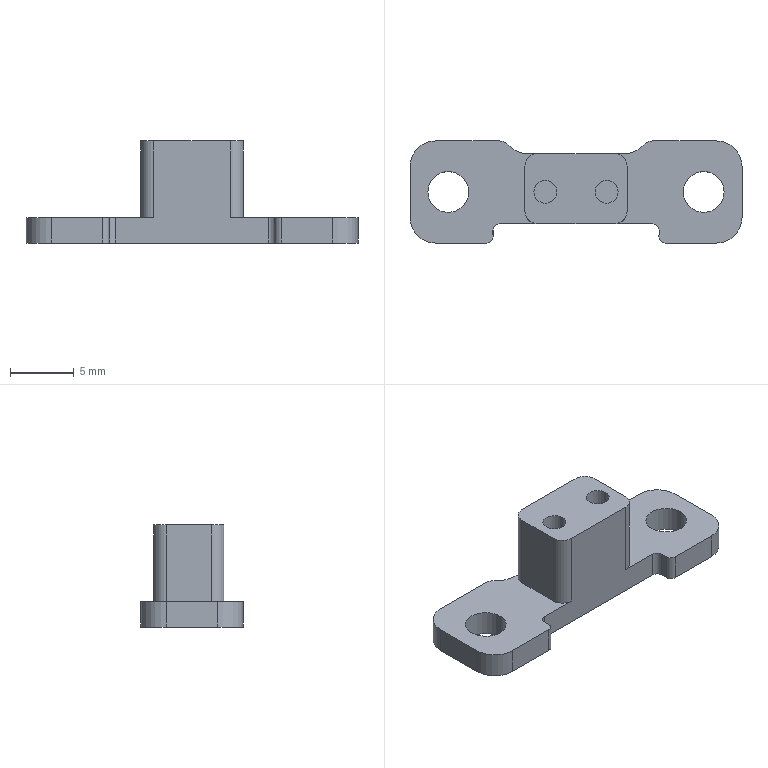Part | 1 solid | 42 faces | volume 546.158 mm3 | cylinder 24 | plane 18 | commonest cylinder face diameters 2 x6 4 x6 1 x4 1.8 x4 3.2 x4